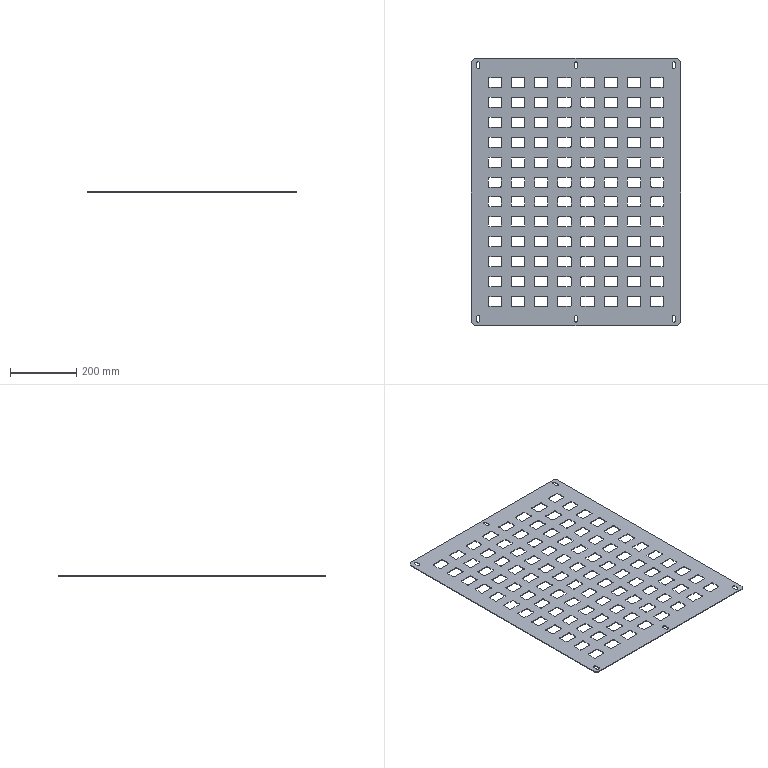Part | STEP file | VD-SYL0380DJ1006_1-5_VD-SYL0380 | 1 solid | 802 faces | box 630 x 805 x 2 mm | volume 782388 mm3 | plane 406 | cylinder 396 | commonest cylinder face diameters 5 x384 10 x12